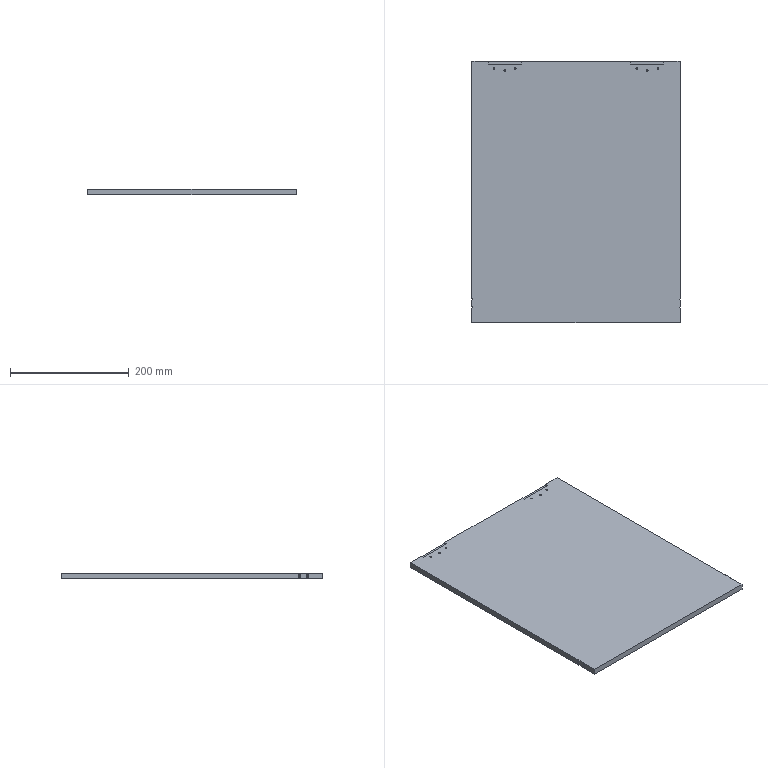Part | SolidWorks | features BaseBody 1 | 1 solid | 58 faces | box 350 x 440 x 10 mm | volume 1538465 mm3 | cylinder 36 | plane 22 | commonest cylinder face diameters 2.5 x24 10 x12